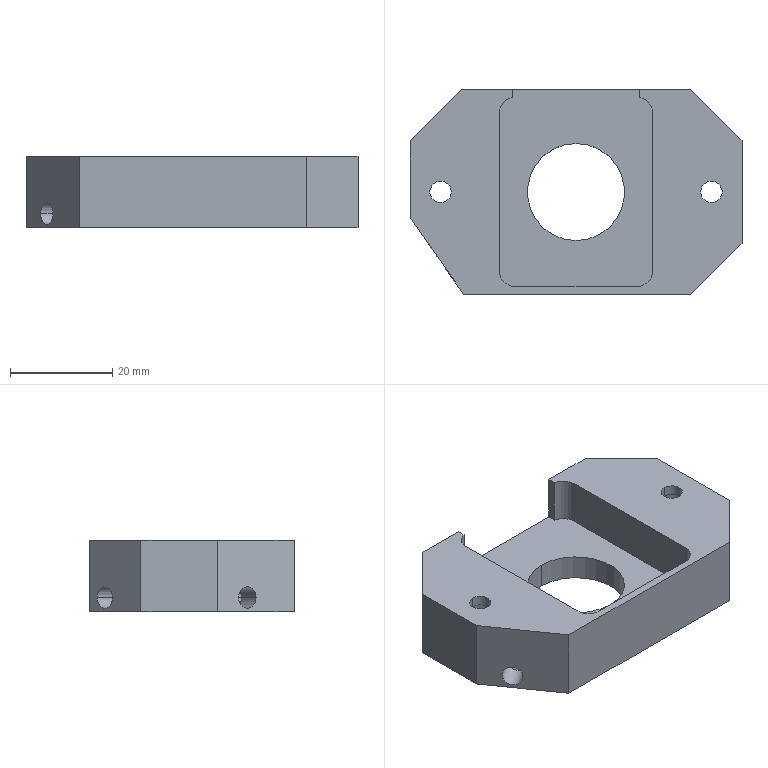Part | 1 solid | 88 faces | box 65 x 40 x 14 mm | volume 18851 mm3 | cylinder 49 | plane 21 | cone 18 | commonest cylinder face diameters 2.05 x12 4.2 x10 2 x8 6 x4 8 x4 3 x3